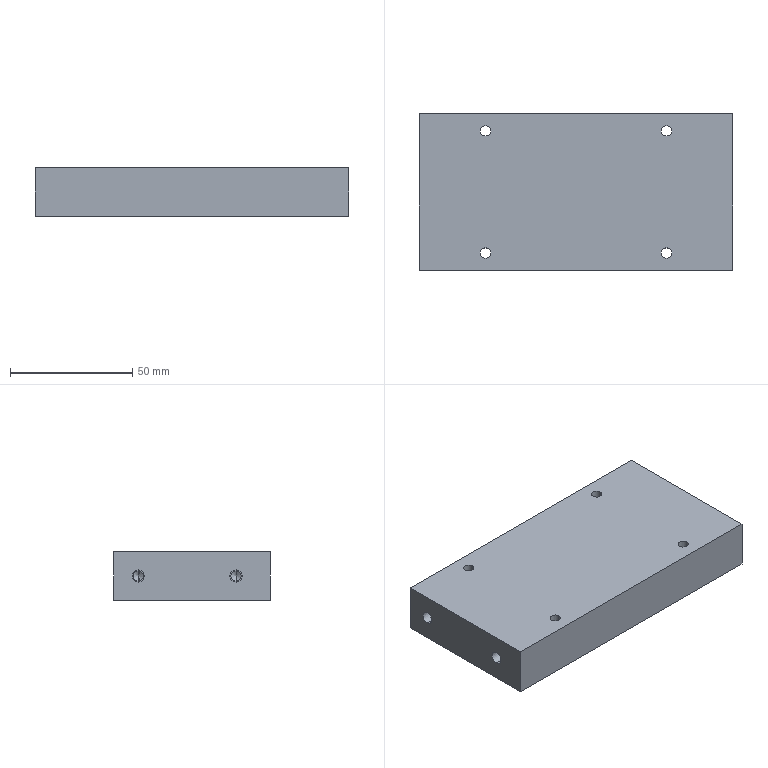Part | SolidWorks | features HoleWzd 2, MirrorPattern 2, Extrusion 1, LPattern 1 | 1 solid | 42 faces | box 128 x 64 x 20 mm | volume 161397 mm3 | cylinder 24 | plane 10 | cone 8 | commonest cylinder face diameters 4.2 x16 5 x8
STEP:
#1=CARTESIAN_POINT('',(109.338,14.,10.));
#2=VERTEX_POINT('',#1);
#3=CARTESIAN_POINT('',(110.6,14.,7.9));
#4=VERTEX_POINT('',#3);
#5=CARTESIAN_POINT('',(110.6,14.,7.9));
#6=DIRECTION('',(0.515,0.,-0.8572));
#7=VECTOR('',#6,1000.);
#8=LINE('',#5,#7);
#9=EDGE_CURVE('',#2,#4,#8,.T.);
#10=ORIENTED_EDGE('',*,*,#9,.F.);
#11=CARTESIAN_POINT('',(110.6,14.,12.1));
#12=VERTEX_POINT('',#11);
#13=CARTESIAN_POINT('',(110.6,14.,12.1));
#14=DIRECTION('',(0.515,0.,0.8572));
#15=VECTOR('',#14,1000.);
#16=LINE('',#13,#15);
#17=EDGE_CURVE('',#2,#12,#16,.T.);
#18=ORIENTED_EDGE('',*,*,#17,.T.);
#19=CARTESIAN_POINT('',(110.6,14.,10.));
#20=DIRECTION('',(1.,0.,0.));
#21=DIRECTION('',(0.,0.,-1.));
#22=AXIS2_PLACEMENT_3D('',#19,#20,#21);
#23=CIRCLE('',#22,2.1);
#24=EDGE_CURVE('',#12,#4,#23,.T.);
#25=ORIENTED_EDGE('',*,*,#24,.T.);
#26=EDGE_LOOP('',(#10,#18,#25));
#27=FACE_OUTER_BOUND('',#26,.T.);
#28=CARTESIAN_POINT('',(110.6,14.,10.));
#29=DIRECTION('',(1.,0.,0.));
#30=DIRECTION('',(0.,0.,-1.));
#31=AXIS2_PLACEMENT_3D('',#28,#29,#30);
#32=CONICAL_SURFACE('',#31,2.1,1.03);
#33=ADVANCED_FACE('',(#27),#32,.F.);
#34=ORIENTED_EDGE('',*,*,#24,.F.);
#35=CARTESIAN_POINT('',(113.,14.,12.1));
#36=VERTEX_POINT('',#35);
#37=CARTESIAN_POINT('',(128.,14.,12.1));
#38=DIRECTION('',(1.,0.,0.));
#39=VECTOR('',#38,1000.);
#40=LINE('',#37,#39);
#41=EDGE_CURVE('',#12,#36,#40,.T.);
#42=ORIENTED_EDGE('',*,*,#41,.T.);
#43=CARTESIAN_POINT('',(113.,14.,7.9));
#44=VERTEX_POINT('',#43);
#45=CARTESIAN_POINT('',(113.,14.,10.));
#46=DIRECTION('',(1.,0.,0.));
#47=DIRECTION('',(0.,0.,-1.));
#48=AXIS2_PLACEMENT_3D('',#45,#46,#47);
#49=CIRCLE('',#48,2.1);
#50=EDGE_CURVE('',#36,#44,#49,.T.);
#51=ORIENTED_EDGE('',*,*,#50,.T.);
#52=CARTESIAN_POINT('',(128.,14.,7.9));
#53=DIRECTION('',(1.,0.,0.));
#54=VECTOR('',#53,1000.);
#55=LINE('',#52,#54);
#56=EDGE_CURVE('',#4,#44,#55,.T.);
#57=ORIENTED_EDGE('',*,*,#56,.F.);
#58=EDGE_LOOP('',(#34,#42,#51,#57));
#59=FACE_OUTER_BOUND('',#58,.T.);
#60=CARTESIAN_POINT('',(128.,14.,10.));
#61=DIRECTION('',(1.,0.,0.));
#62=DIRECTION('',(0.,0.,-1.));
#63=AXIS2_PLACEMENT_3D('',#60,#61,#62);
#64=CYLINDRICAL_SURFACE('',#63,2.1);
#65=ADVANCED_FACE('',(#59),#64,.F.);
#66=CARTESIAN_POINT('',(113.,14.,12.5));
#67=VERTEX_POINT('',#66);
#68=CARTESIAN_POINT('',(113.,14.,7.5));
#69=VERTEX_POINT('',#68);
#70=CARTESIAN_POINT('',(113.,14.,10.));
#71=DIRECTION('',(1.,0.,0.));
#72=DIRECTION('',(0.,0.,-1.));
#73=AXIS2_PLACEMENT_3D('',#70,#71,#72);
#74=CIRCLE('',#73,2.5);
#75=EDGE_CURVE('',#67,#69,#74,.T.);
#76=ORIENTED_EDGE('',*,*,#75,.F.);
#77=CARTESIAN_POINT('',(128.,14.,12.5));
#78=VERTEX_POINT('',#77);
#79=CARTESIAN_POINT('',(128.,14.,12.5));
#80=DIRECTION('',(1.,0.,0.));
#81=VECTOR('',#80,1000.);
#82=LINE('',#79,#81);
#83=EDGE_CURVE('',#67,#78,#82,.T.);
#84=ORIENTED_EDGE('',*,*,#83,.T.);
#85=CARTESIAN_POINT('',(128.,14.,7.5));
#86=VERTEX_POINT('',#85);
#87=CARTESIAN_POINT('',(128.,14.,10.));
#88=DIRECTION('',(1.,0.,0.));
#89=DIRECTION('',(0.,0.,-1.));
#90=AXIS2_PLACEMENT_3D('',#87,#88,#89);
#91=CIRCLE('',#90,2.5);
#92=EDGE_CURVE('',#78,#86,#91,.T.);
#93=ORIENTED_EDGE('',*,*,#92,.T.);
#94=CARTESIAN_POINT('',(128.,14.,7.5));
#95=DIRECTION('',(1.,0.,0.));
#96=VECTOR('',#95,1000.);
#97=LINE('',#94,#96);
#98=EDGE_CURVE('',#69,#86,#97,.T.);
#99=ORIENTED_EDGE('',*,*,#98,.F.);
#100=EDGE_LOOP('',(#76,#84,#93,#99));
#101=FACE_OUTER_BOUND('',#100,.T.);
#102=CARTESIAN_POINT('',(128.,14.,10.));
#103=DIRECTION('',(1.,0.,0.));
#104=DIRECTION('',(0.,0.,-1.));
#105=AXIS2_PLACEMENT_3D('',#102,#103,#104);
#106=CYLINDRICAL_SURFACE('',#105,2.5);
#107=ADVANCED_FACE('',(#101),#106,.F.);
#108=CARTESIAN_POINT('',(18.662,14.,10.));
#109=VERTEX_POINT('',#108);
#110=CARTESIAN_POINT('',(17.4,14.,12.1));
#111=VERTEX_POINT('',#110);
#112=CARTESIAN_POINT('',(17.4,14.,12.1));
#113=DIRECTION('',(-0.515,0.,0.8572));
#114=VECTOR('',#113,1000.);
#115=LINE('',#112,#114);
#116=EDGE_CURVE('',#109,#111,#115,.T.);
#117=ORIENTED_EDGE('',*,*,#116,.F.);
#118=CARTESIAN_POINT('',(17.4,14.,7.9));
#119=VERTEX_POINT('',#118);
#120=CARTESIAN_POINT('',(17.4,14.,7.9));
#121=DIRECTION('',(-0.515,0.,-0.8572));
#122=VECTOR('',#121,1000.);
#123=LINE('',#120,#122);
#124=EDGE_CURVE('',#109,#119,#123,.T.);
#125=ORIENTED_EDGE('',*,*,#124,.T.);
#126=CARTESIAN_POINT('',(17.4,14.,10.));
#127=DIRECTION('',(-1.,0.,0.));
#128=DIRECTION('',(0.,0.,1.));
#129=AXIS2_PLACEMENT_3D('',#126,#127,#128);
#130=CIRCLE('',#129,2.1);
#131=EDGE_CURVE('',#119,#111,#130,.T.);
#132=ORIENTED_EDGE('',*,*,#131,.T.);
#133=EDGE_LOOP('',(#117,#125,#132));
#134=FACE_OUTER_BOUND('',#133,.T.);
#135=CARTESIAN_POINT('',(17.4,14.,10.));
#136=DIRECTION('',(-1.,0.,0.));
#137=DIRECTION('',(0.,0.,1.));
#138=AXIS2_PLACEMENT_3D('',#135,#136,#137);
#139=CONICAL_SURFACE('',#138,2.1,1.03);
#140=ADVANCED_FACE('',(#134),#139,.F.);
#141=ORIENTED_EDGE('',*,*,#131,.F.);
#142=CARTESIAN_POINT('',(15.,14.,7.9));
#143=VERTEX_POINT('',#142);
#144=CARTESIAN_POINT('',(0.,14.,7.9));
#145=DIRECTION('',(-1.,0.,0.));
#146=VECTOR('',#145,1000.);
#147=LINE('',#144,#146);
#148=EDGE_CURVE('',#119,#143,#147,.T.);
#149=ORIENTED_EDGE('',*,*,#148,.T.);
#150=CARTESIAN_POINT('',(15.,14.,12.1));
#151=VERTEX_POINT('',#150);
#152=CARTESIAN_POINT('',(15.,14.,10.));
#153=DIRECTION('',(-1.,0.,0.));
#154=DIRECTION('',(0.,0.,1.));
#155=AXIS2_PLACEMENT_3D('',#152,#153,#154);
#156=CIRCLE('',#155,2.1);
#157=EDGE_CURVE('',#143,#151,#156,.T.);
#158=ORIENTED_EDGE('',*,*,#157,.T.);
#159=CARTESIAN_POINT('',(0.,14.,12.1));
#160=DIRECTION('',(-1.,0.,0.));
#161=VECTOR('',#160,1000.);
#162=LINE('',#159,#161);
#163=EDGE_CURVE('',#111,#151,#162,.T.);
#164=ORIENTED_EDGE('',*,*,#163,.F.);
#165=EDGE_LOOP('',(#141,#149,#158,#164));
#166=FACE_OUTER_BOUND('',#165,.T.);
#167=CARTESIAN_POINT('',(0.,14.,10.));
#168=DIRECTION('',(-1.,0.,0.));
#169=DIRECTION('',(0.,0.,1.));
#170=AXIS2_PLACEMENT_3D('',#167,#168,#169);
#171=CYLINDRICAL_SURFACE('',#170,2.1);
#172=ADVANCED_FACE('',(#166),#171,.F.);
#173=CARTESIAN_POINT('',(15.,14.,7.5));
#174=VERTEX_POINT('',#173);
#175=CARTESIAN_POINT('',(15.,14.,12.5));
#176=VERTEX_POINT('',#175);
#177=CARTESIAN_POINT('',(15.,14.,10.));
#178=DIRECTION('',(-1.,0.,0.));
#179=DIRECTION('',(0.,0.,1.));
#180=AXIS2_PLACEMENT_3D('',#177,#178,#179);
#181=CIRCLE('',#180,2.5);
#182=EDGE_CURVE('',#174,#176,#181,.T.);
#183=ORIENTED_EDGE('',*,*,#182,.F.);
#184=CARTESIAN_POINT('',(0.,14.,7.5));
#185=VERTEX_POINT('',#184);
#186=CARTESIAN_POINT('',(0.,14.,7.5));
#187=DIRECTION('',(-1.,0.,0.));
#188=VECTOR('',#187,1000.);
#189=LINE('',#186,#188);
#190=EDGE_CURVE('',#174,#185,#189,.T.);
#191=ORIENTED_EDGE('',*,*,#190,.T.);
#192=CARTESIAN_POINT('',(0.,14.,12.5));
#193=VERTEX_POINT('',#192);
#194=CARTESIAN_POINT('',(0.,14.,10.));
#195=DIRECTION('',(-1.,0.,0.));
#196=DIRECTION('',(0.,0.,1.));
#197=AXIS2_PLACEMENT_3D('',#194,#195,#196);
#198=CIRCLE('',#197,2.5);
#199=EDGE_CURVE('',#185,#193,#198,.T.);
#200=ORIENTED_EDGE('',*,*,#199,.T.);
#201=CARTESIAN_POINT('',(0.,14.,12.5));
#202=DIRECTION('',(-1.,0.,0.));
#203=VECTOR('',#202,1000.);
#204=LINE('',#201,#203);
#205=EDGE_CURVE('',#176,#193,#204,.T.);
#206=ORIENTED_EDGE('',*,*,#205,.F.);
#207=EDGE_LOOP('',(#183,#191,#200,#206));
#208=FACE_OUTER_BOUND('',#207,.T.);
#209=CARTESIAN_POINT('',(0.,14.,10.));
#210=DIRECTION('',(-1.,0.,0.));
#211=DIRECTION('',(0.,0.,1.));
#212=AXIS2_PLACEMENT_3D('',#209,#210,#211);
#213=CYLINDRICAL_SURFACE('',#212,2.5);
#214=ADVANCED_FACE('',(#208),#213,.F.);
#215=CARTESIAN_POINT('',(109.338,54.,10.));
#216=VERTEX_POINT('',#215);
#217=CARTESIAN_POINT('',(110.6,54.,7.9));
#218=VERTEX_POINT('',#217);
#219=CARTESIAN_POINT('',(110.6,54.,7.9));
#220=DIRECTION('',(0.515,0.,-0.8572));
#221=VECTOR('',#220,1000.);
#222=LINE('',#219,#221);
#223=EDGE_CURVE('',#216,#218,#222,.T.);
#224=ORIENTED_EDGE('',*,*,#223,.F.);
#225=CARTESIAN_POINT('',(110.6,54.,12.1));
#226=VERTEX_POINT('',#225);
#227=CARTESIAN_POINT('',(110.6,54.,12.1));
#228=DIRECTION('',(0.515,0.,0.8572));
#229=VECTOR('',#228,1000.);
#230=LINE('',#227,#229);
#231=EDGE_CURVE('',#216,#226,#230,.T.);
#232=ORIENTED_EDGE('',*,*,#231,.T.);
#233=CARTESIAN_POINT('',(110.6,54.,10.));
#234=DIRECTION('',(1.,0.,0.));
#235=DIRECTION('',(0.,0.,-1.));
#236=AXIS2_PLACEMENT_3D('',#233,#234,#235);
#237=CIRCLE('',#236,2.1);
#238=EDGE_CURVE('',#226,#218,#237,.T.);
#239=ORIENTED_EDGE('',*,*,#238,.T.);
#240=EDGE_LOOP('',(#224,#232,#239));
#241=FACE_OUTER_BOUND('',#240,.T.);
#242=CARTESIAN_POINT('',(110.6,54.,10.));
#243=DIRECTION('',(1.,0.,0.));
#244=DIRECTION('',(0.,0.,-1.));
#245=AXIS2_PLACEMENT_3D('',#242,#243,#244);
#246=CONICAL_SURFACE('',#245,2.1,1.03);
#247=ADVANCED_FACE('',(#241),#246,.F.);
#248=ORIENTED_EDGE('',*,*,#238,.F.);
#249=CARTESIAN_POINT('',(113.,54.,12.1));
#250=VERTEX_POINT('',#249);
#251=CARTESIAN_POINT('',(128.,54.,12.1));
#252=DIRECTION('',(1.,0.,0.));
#253=VECTOR('',#252,1000.);
#254=LINE('',#251,#253);
#255=EDGE_CURVE('',#226,#250,#254,.T.);
#256=ORIENTED_EDGE('',*,*,#255,.T.);
#257=CARTESIAN_POINT('',(113.,54.,7.9));
#258=VERTEX_POINT('',#257);
#259=CARTESIAN_POINT('',(113.,54.,10.));
#260=DIRECTION('',(1.,0.,0.));
#261=DIRECTION('',(0.,0.,-1.));
#262=AXIS2_PLACEMENT_3D('',#259,#260,#261);
#263=CIRCLE('',#262,2.1);
#264=EDGE_CURVE('',#250,#258,#263,.T.);
#265=ORIENTED_EDGE('',*,*,#264,.T.);
#266=CARTESIAN_POINT('',(128.,54.,7.9));
#267=DIRECTION('',(1.,0.,0.));
#268=VECTOR('',#267,1000.);
#269=LINE('',#266,#268);
#270=EDGE_CURVE('',#218,#258,#269,.T.);
#271=ORIENTED_EDGE('',*,*,#270,.F.);
#272=EDGE_LOOP('',(#248,#256,#265,#271));
#273=FACE_OUTER_BOUND('',#272,.T.);
#274=CARTESIAN_POINT('',(128.,54.,10.));
#275=DIRECTION('',(1.,0.,0.));
#276=DIRECTION('',(0.,0.,-1.));
#277=AXIS2_PLACEMENT_3D('',#274,#275,#276);
#278=CYLINDRICAL_SURFACE('',#277,2.1);
#279=ADVANCED_FACE('',(#273),#278,.F.);
#280=CARTESIAN_POINT('',(113.,54.,12.5));
#281=VERTEX_POINT('',#280);
#282=CARTESIAN_POINT('',(113.,54.,7.5));
#283=VERTEX_POINT('',#282);
#284=CARTESIAN_POINT('',(113.,54.,10.));
#285=DIRECTION('',(1.,0.,0.));
#286=DIRECTION('',(0.,0.,-1.));
#287=AXIS2_PLACEMENT_3D('',#284,#285,#286);
#288=CIRCLE('',#287,2.5);
#289=EDGE_CURVE('',#281,#283,#288,.T.);
#290=ORIENTED_EDGE('',*,*,#289,.F.);
#291=CARTESIAN_POINT('',(128.,54.,12.5));
#292=VERTEX_POINT('',#291);
#293=CARTESIAN_POINT('',(128.,54.,12.5));
#294=DIRECTION('',(1.,0.,0.));
#295=VECTOR('',#294,1000.);
#296=LINE('',#293,#295);
#297=EDGE_CURVE('',#281,#292,#296,.T.);
#298=ORIENTED_EDGE('',*,*,#297,.T.);
#299=CARTESIAN_POINT('',(128.,54.,7.5));
#300=VERTEX_POINT('',#299);
#301=CARTESIAN_POINT('',(128.,54.,10.));
#302=DIRECTION('',(1.,0.,0.));
#303=DIRECTION('',(0.,0.,-1.));
#304=AXIS2_PLACEMENT_3D('',#301,#302,#303);
#305=CIRCLE('',#304,2.5);
#306=EDGE_CURVE('',#292,#300,#305,.T.);
#307=ORIENTED_EDGE('',*,*,#306,.T.);
#308=CARTESIAN_POINT('',(128.,54.,7.5));
#309=DIRECTION('',(1.,0.,0.));
#310=VECTOR('',#309,1000.);
#311=LINE('',#308,#310);
#312=EDGE_CURVE('',#283,#300,#311,.T.);
#313=ORIENTED_EDGE('',*,*,#312,.F.);
#314=EDGE_LOOP('',(#290,#298,#307,#313));
#315=FACE_OUTER_BOUND('',#314,.T.);
#316=CARTESIAN_POINT('',(128.,54.,10.));
#317=DIRECTION('',(1.,0.,0.));
#318=DIRECTION('',(0.,0.,-1.));
#319=AXIS2_PLACEMENT_3D('',#316,#317,#318);
#320=CYLINDRICAL_SURFACE('',#319,2.5);
#321=ADVANCED_FACE('',(#315),#320,.F.);
#322=CARTESIAN_POINT('',(18.662,54.,10.));
#323=VERTEX_POINT('',#322);
#324=CARTESIAN_POINT('',(17.4,54.,12.1));
#325=VERTEX_POINT('',#324);
#326=CARTESIAN_POINT('',(17.4,54.,12.1));
#327=DIRECTION('',(-0.515,0.,0.8572));
#328=VECTOR('',#327,1000.);
#329=LINE('',#326,#328);
#330=EDGE_CURVE('',#323,#325,#329,.T.);
#331=ORIENTED_EDGE('',*,*,#330,.F.);
#332=CARTESIAN_POINT('',(17.4,54.,7.9));
#333=VERTEX_POINT('',#332);
#334=CARTESIAN_POINT('',(17.4,54.,7.9));
#335=DIRECTION('',(-0.515,0.,-0.8572));
#336=VECTOR('',#335,1000.);
#337=LINE('',#334,#336);
#338=EDGE_CURVE('',#323,#333,#337,.T.);
#339=ORIENTED_EDGE('',*,*,#338,.T.);
#340=CARTESIAN_POINT('',(17.4,54.,10.));
#341=DIRECTION('',(-1.,0.,0.));
#342=DIRECTION('',(0.,0.,1.));
#343=AXIS2_PLACEMENT_3D('',#340,#341,#342);
#344=CIRCLE('',#343,2.1);
#345=EDGE_CURVE('',#333,#325,#344,.T.);
#346=ORIENTED_EDGE('',*,*,#345,.T.);
#347=EDGE_LOOP('',(#331,#339,#346));
#348=FACE_OUTER_BOUND('',#347,.T.);
#349=CARTESIAN_POINT('',(17.4,54.,10.));
#350=DIRECTION('',(-1.,0.,0.));
#351=DIRECTION('',(0.,0.,1.));
#352=AXIS2_PLACEMENT_3D('',#349,#350,#351);
#353=CONICAL_SURFACE('',#352,2.1,1.03);
#354=ADVANCED_FACE('',(#348),#353,.F.);
#355=ORIENTED_EDGE('',*,*,#345,.F.);
#356=CARTESIAN_POINT('',(15.,54.,7.9));
#357=VERTEX_POINT('',#356);
#358=CARTESIAN_POINT('',(0.,54.,7.9));
#359=DIRECTION('',(-1.,0.,0.));
#360=VECTOR('',#359,1000.);
#361=LINE('',#358,#360);
#362=EDGE_CURVE('',#333,#357,#361,.T.);
#363=ORIENTED_EDGE('',*,*,#362,.T.);
#364=CARTESIAN_POINT('',(15.,54.,12.1));
#365=VERTEX_POINT('',#364);
#366=CARTESIAN_POINT('',(15.,54.,10.));
#367=DIRECTION('',(-1.,0.,0.));
#368=DIRECTION('',(0.,0.,1.));
#369=AXIS2_PLACEMENT_3D('',#366,#367,#368);
#370=CIRCLE('',#369,2.1);
#371=EDGE_CURVE('',#357,#365,#370,.T.);
#372=ORIENTED_EDGE('',*,*,#371,.T.);
#373=CARTESIAN_POINT('',(0.,54.,12.1));
#374=DIRECTION('',(-1.,0.,0.));
#375=VECTOR('',#374,1000.);
#376=LINE('',#373,#375);
#377=EDGE_CURVE('',#325,#365,#376,.T.);
#378=ORIENTED_EDGE('',*,*,#377,.F.);
#379=EDGE_LOOP('',(#355,#363,#372,#378));
#380=FACE_OUTER_BOUND('',#379,.T.);
#381=CARTESIAN_POINT('',(0.,54.,10.));
#382=DIRECTION('',(-1.,0.,0.));
#383=DIRECTION('',(0.,0.,1.));
#384=AXIS2_PLACEMENT_3D('',#381,#382,#383);
#385=CYLINDRICAL_SURFACE('',#384,2.1);
#386=ADVANCED_FACE('',(#380),#385,.F.);
#387=CARTESIAN_POINT('',(15.,54.,7.5));
#388=VERTEX_POINT('',#387);
#389=CARTESIAN_POINT('',(15.,54.,12.5));
#390=VERTEX_POINT('',#389);
#391=CARTESIAN_POINT('',(15.,54.,10.));
#392=DIRECTION('',(-1.,0.,0.));
#393=DIRECTION('',(0.,0.,1.));
#394=AXIS2_PLACEMENT_3D('',#391,#392,#393);
#395=CIRCLE('',#394,2.5);
#396=EDGE_CURVE('',#388,#390,#395,.T.);
#397=ORIENTED_EDGE('',*,*,#396,.F.);
#398=CARTESIAN_POINT('',(0.,54.,7.5));
#399=VERTEX_POINT('',#398);
#400=CARTESIAN_POINT('',(0.,54.,7.5));
#401=DIRECTION('',(-1.,0.,0.));
#402=VECTOR('',#401,1000.);
#403=LINE('',#400,#402);
#404=EDGE_CURVE('',#388,#399,#403,.T.);
#405=ORIENTED_EDGE('',*,*,#404,.T.);
#406=CARTESIAN_POINT('',(0.,54.,12.5));
#407=VERTEX_POINT('',#406);
#408=CARTESIAN_POINT('',(0.,54.,10.));
#409=DIRECTION('',(-1.,0.,0.));
#410=DIRECTION('',(0.,0.,1.));
#411=AXIS2_PLACEMENT_3D('',#408,#409,#410);
#412=CIRCLE('',#411,2.5);
#413=EDGE_CURVE('',#399,#407,#412,.T.);
#414=ORIENTED_EDGE('',*,*,#413,.T.);
#415=CARTESIAN_POINT('',(0.,54.,12.5));
#416=DIRECTION('',(-1.,0.,0.));
#417=VECTOR('',#416,1000.);
#418=LINE('',#415,#417);
#419=EDGE_CURVE('',#390,#407,#418,.T.);
#420=ORIENTED_EDGE('',*,*,#419,.F.);
#421=EDGE_LOOP('',(#397,#405,#414,#420));
#422=FACE_OUTER_BOUND('',#421,.T.);
#423=CARTESIAN_POINT('',(0.,54.,10.));
#424=DIRECTION('',(-1.,0.,0.));
#425=DIRECTION('',(0.,0.,1.));
#426=AXIS2_PLACEMENT_3D('',#423,#424,#425);
#427=CYLINDRICAL_SURFACE('',#426,2.5);
#428=ADVANCED_FACE('',(#422),#427,.F.);
#429=CARTESIAN_POINT('',(24.9,57.,0.));
#430=VERTEX_POINT('',#429);
#431=CARTESIAN_POINT('',(29.1,57.,0.));
#432=VERTEX_POINT('',#431);
#433=CARTESIAN_POINT('',(27.,57.,0.));
#434=DIRECTION('',(0.,0.,1.));
#435=DIRECTION('',(1.,0.,0.));
#436=AXIS2_PLACEMENT_3D('',#433,#434,#435);
#437=CIRCLE('',#436,2.1);
#438=EDGE_CURVE('',#430,#432,#437,.T.);
#439=ORIENTED_EDGE('',*,*,#438,.F.);
#440=CARTESIAN_POINT('',(24.9,57.,20.));
#441=VERTEX_POINT('',#440);
#442=CARTESIAN_POINT('',(24.9,57.,20.));
#443=DIRECTION('',(0.,0.,1.));
#444=VECTOR('',#443,1000.);
#445=LINE('',#442,#444);
#446=EDGE_CURVE('',#430,#441,#445,.T.);
#447=ORIENTED_EDGE('',*,*,#446,.T.);
#448=CARTESIAN_POINT('',(29.1,57.,20.));
#449=VERTEX_POINT('',#448);
#450=CARTESIAN_POINT('',(27.,57.,20.));
#451=DIRECTION('',(0.,0.,1.));
#452=DIRECTION('',(1.,0.,0.));
#453=AXIS2_PLACEMENT_3D('',#450,#451,#452);
#454=CIRCLE('',#453,2.1);
#455=EDGE_CURVE('',#441,#449,#454,.T.);
#456=ORIENTED_EDGE('',*,*,#455,.T.);
#457=CARTESIAN_POINT('',(29.1,57.,20.));
#458=DIRECTION('',(0.,0.,1.));
#459=VECTOR('',#458,1000.);
#460=LINE('',#457,#459);
#461=EDGE_CURVE('',#432,#449,#460,.T.);
#462=ORIENTED_EDGE('',*,*,#461,.F.);
#463=EDGE_LOOP('',(#439,#447,#456,#462));
#464=FACE_OUTER_BOUND('',#463,.T.);
#465=CARTESIAN_POINT('',(27.,57.,20.));
#466=DIRECTION('',(0.,0.,1.));
#467=DIRECTION('',(1.,0.,0.));
#468=AXIS2_PLACEMENT_3D('',#465,#466,#467);
#469=CYLINDRICAL_SURFACE('',#468,2.1);
#470=ADVANCED_FACE('',(#464),#469,.F.);
#471=CARTESIAN_POINT('',(24.9,7.,0.));
#472=VERTEX_POINT('',#471);
#473=CARTESIAN_POINT('',(29.1,7.,0.));
#474=VERTEX_POINT('',#473);
#475=CARTESIAN_POINT('',(27.,7.,0.));
#476=DIRECTION('',(0.,0.,1.));
#477=DIRECTION('',(1.,0.,0.));
#478=AXIS2_PLACEMENT_3D('',#475,#476,#477);
#479=CIRCLE('',#478,2.1);
#480=EDGE_CURVE('',#472,#474,#479,.T.);
#481=ORIENTED_EDGE('',*,*,#480,.F.);
#482=CARTESIAN_POINT('',(24.9,7.,20.));
#483=VERTEX_POINT('',#482);
#484=CARTESIAN_POINT('',(24.9,7.,20.));
#485=DIRECTION('',(0.,0.,1.));
#486=VECTOR('',#485,1000.);
#487=LINE('',#484,#486);
#488=EDGE_CURVE('',#472,#483,#487,.T.);
#489=ORIENTED_EDGE('',*,*,#488,.T.);
#490=CARTESIAN_POINT('',(29.1,7.,20.));
#491=VERTEX_POINT('',#490);
#492=CARTESIAN_POINT('',(27.,7.,20.));
#493=DIRECTION('',(0.,0.,1.));
#494=DIRECTION('',(1.,0.,0.));
#495=AXIS2_PLACEMENT_3D('',#492,#493,#494);
#496=CIRCLE('',#495,2.1);
#497=EDGE_CURVE('',#483,#491,#496,.T.);
#498=ORIENTED_EDGE('',*,*,#497,.T.);
#499=CARTESIAN_POINT('',(29.1,7.,20.));
#500=DIRECTION('',(0.,0.,1.));
#501=VECTOR('',#500,1000.);
#502=LINE('',#499,#501);
#503=EDGE_CURVE('',#474,#491,#502,.T.);
#504=ORIENTED_EDGE('',*,*,#503,.F.);
#505=EDGE_LOOP('',(#481,#489,#498,#504));
#506=FACE_OUTER_BOUND('',#505,.T.);
#507=CARTESIAN_POINT('',(27.,7.,20.));
#508=DIRECTION('',(0.,0.,1.));
#509=DIRECTION('',(1.,0.,0.));
#510=AXIS2_PLACEMENT_3D('',#507,#508,#509);
#511=CYLINDRICAL_SURFACE('',#510,2.1);
#512=ADVANCED_FACE('',(#506),#511,.F.);
#513=CARTESIAN_POINT('',(98.9,7.,0.));
#514=VERTEX_POINT('',#513);
#515=CARTESIAN_POINT('',(103.1,7.,0.));
#516=VERTEX_POINT('',#515);
#517=CARTESIAN_POINT('',(101.,7.,0.));
#518=DIRECTION('',(0.,0.,1.));
#519=DIRECTION('',(1.,0.,0.));
#520=AXIS2_PLACEMENT_3D('',#517,#518,#519);
#521=CIRCLE('',#520,2.1);
#522=EDGE_CURVE('',#514,#516,#521,.T.);
#523=ORIENTED_EDGE('',*,*,#522,.F.);
#524=CARTESIAN_POINT('',(98.9,7.,20.));
#525=VERTEX_POINT('',#524);
#526=CARTESIAN_POINT('',(98.9,7.,20.));
#527=DIRECTION('',(0.,0.,1.));
#528=VECTOR('',#527,1000.);
#529=LINE('',#526,#528);
#530=EDGE_CURVE('',#514,#525,#529,.T.);
#531=ORIENTED_EDGE('',*,*,#530,.T.);
#532=CARTESIAN_POINT('',(103.1,7.,20.));
#533=VERTEX_POINT('',#532);
#534=CARTESIAN_POINT('',(101.,7.,20.));
#535=DIRECTION('',(0.,0.,1.));
#536=DIRECTION('',(1.,0.,0.));
#537=AXIS2_PLACEMENT_3D('',#534,#535,#536);
#538=CIRCLE('',#537,2.1);
#539=EDGE_CURVE('',#525,#533,#538,.T.);
#540=ORIENTED_EDGE('',*,*,#539,.T.);
#541=CARTESIAN_POINT('',(103.1,7.,20.));
#542=DIRECTION('',(0.,0.,1.));
#543=VECTOR('',#542,1000.);
#544=LINE('',#541,#543);
#545=EDGE_CURVE('',#516,#533,#544,.T.);
#546=ORIENTED_EDGE('',*,*,#545,.F.);
#547=EDGE_LOOP('',(#523,#531,#540,#546));
#548=FACE_OUTER_BOUND('',#547,.T.);
#549=CARTESIAN_POINT('',(101.,7.,20.));
#550=DIRECTION('',(0.,0.,1.));
#551=DIRECTION('',(1.,0.,0.));
#552=AXIS2_PLACEMENT_3D('',#549,#550,#551);
#553=CYLINDRICAL_SURFACE('',#552,2.1);
#554=ADVANCED_FACE('',(#548),#553,.F.);
#555=CARTESIAN_POINT('',(98.9,57.,0.));
#556=VERTEX_POINT('',#555);
#557=CARTESIAN_POINT('',(103.1,57.,0.));
#558=VERTEX_POINT('',#557);
#559=CARTESIAN_POINT('',(101.,57.,0.));
#560=DIRECTION('',(0.,0.,1.));
#561=DIRECTION('',(1.,0.,0.));
#562=AXIS2_PLACEMENT_3D('',#559,#560,#561);
#563=CIRCLE('',#562,2.1);
#564=EDGE_CURVE('',#556,#558,#563,.T.);
#565=ORIENTED_EDGE('',*,*,#564,.F.);
#566=CARTESIAN_POINT('',(98.9,57.,20.));
#567=VERTEX_POINT('',#566);
#568=CARTESIAN_POINT('',(98.9,57.,20.));
#569=DIRECTION('',(0.,0.,1.));
#570=VECTOR('',#569,1000.);
#571=LINE('',#568,#570);
#572=EDGE_CURVE('',#556,#567,#571,.T.);
#573=ORIENTED_EDGE('',*,*,#572,.T.);
#574=CARTESIAN_POINT('',(103.1,57.,20.));
#575=VERTEX_POINT('',#574);
#576=CARTESIAN_POINT('',(101.,57.,20.));
#577=DIRECTION('',(0.,0.,1.));
#578=DIRECTION('',(1.,0.,0.));
#579=AXIS2_PLACEMENT_3D('',#576,#577,#578);
#580=CIRCLE('',#579,2.1);
#581=EDGE_CURVE('',#567,#575,#580,.T.);
#582=ORIENTED_EDGE('',*,*,#581,.T.);
#583=CARTESIAN_POINT('',(103.1,57.,20.));
#584=DIRECTION('',(0.,0.,1.));
#585=VECTOR('',#584,1000.);
#586=LINE('',#583,#585);
#587=EDGE_CURVE('',#558,#575,#586,.T.);
#588=ORIENTED_EDGE('',*,*,#587,.F.);
#589=EDGE_LOOP('',(#565,#573,#582,#588));
#590=FACE_OUTER_BOUND('',#589,.T.);
#591=CARTESIAN_POINT('',(101.,57.,20.));
#592=DIRECTION('',(0.,0.,1.));
#593=DIRECTION('',(1.,0.,0.));
#594=AXIS2_PLACEMENT_3D('',#591,#592,#593);
#595=CYLINDRICAL_SURFACE('',#594,2.1);
#596=ADVANCED_FACE('',(#590),#595,.F.);
#597=CARTESIAN_POINT('',(27.,57.,0.));
#598=DIRECTION('',(0.,0.,1.));
#599=DIRECTION('',(1.,0.,0.));
#600=AXIS2_PLACEMENT_3D('',#597,#598,#599);
#601=CIRCLE('',#600,2.1);
#602=EDGE_CURVE('',#432,#430,#601,.T.);
#603=ORIENTED_EDGE('',*,*,#602,.T.);
#604=ORIENTED_EDGE('',*,*,#438,.T.);
#605=EDGE_LOOP('',(#603,#604));
#606=FACE_BOUND('',#605,.T.);
#607=CARTESIAN_POINT('',(27.,7.,0.));
#608=DIRECTION('',(0.,0.,1.));
#609=DIRECTION('',(1.,0.,0.));
#610=AXIS2_PLACEMENT_3D('',#607,#608,#609);
#611=CIRCLE('',#610,2.1);
#612=EDGE_CURVE('',#474,#472,#611,.T.);
#613=ORIENTED_EDGE('',*,*,#612,.T.);
#614=ORIENTED_EDGE('',*,*,#480,.T.);
#615=EDGE_LOOP('',(#613,#614));
#616=FACE_BOUND('',#615,.T.);
#617=CARTESIAN_POINT('',(101.,7.,0.));
#618=DIRECTION('',(0.,0.,1.));
#619=DIRECTION('',(1.,0.,0.));
#620=AXIS2_PLACEMENT_3D('',#617,#618,#619);
#621=CIRCLE('',#620,2.1);
#622=EDGE_CURVE('',#516,#514,#621,.T.);
#623=ORIENTED_EDGE('',*,*,#622,.T.);
#624=ORIENTED_EDGE('',*,*,#522,.T.);
#625=EDGE_LOOP('',(#623,#624));
#626=FACE_BOUND('',#625,.T.);
#627=CARTESIAN_POINT('',(0.,64.,0.));
#628=VERTEX_POINT('',#627);
#629=CARTESIAN_POINT('',(0.,0.,0.));
#630=VERTEX_POINT('',#629);
#631=CARTESIAN_POINT('',(0.,0.,0.));
#632=DIRECTION('',(0.,-1.,0.));
#633=VECTOR('',#632,1000.);
#634=LINE('',#631,#633);
#635=EDGE_CURVE('',#628,#630,#634,.T.);
#636=ORIENTED_EDGE('',*,*,#635,.F.);
#637=CARTESIAN_POINT('',(128.,64.,0.));
#638=VERTEX_POINT('',#637);
#639=CARTESIAN_POINT('',(0.,64.,0.));
#640=DIRECTION('',(-1.,0.,0.));
#641=VECTOR('',#640,1000.);
#642=LINE('',#639,#641);
#643=EDGE_CURVE('',#638,#628,#642,.T.);
#644=ORIENTED_EDGE('',*,*,#643,.F.);
#645=CARTESIAN_POINT('',(128.,0.,0.));
#646=VERTEX_POINT('',#645);
#647=CARTESIAN_POINT('',(128.,0.,0.));
#648=DIRECTION('',(0.,1.,0.));
#649=VECTOR('',#648,1000.);
#650=LINE('',#647,#649);
#651=EDGE_CURVE('',#646,#638,#650,.T.);
#652=ORIENTED_EDGE('',*,*,#651,.F.);
#653=CARTESIAN_POINT('',(0.,0.,0.));
#654=DIRECTION('',(1.,0.,0.));
#655=VECTOR('',#654,1000.);
#656=LINE('',#653,#655);
#657=EDGE_CURVE('',#630,#646,#656,.T.);
#658=ORIENTED_EDGE('',*,*,#657,.F.);
#659=EDGE_LOOP('',(#636,#644,#652,#658));
#660=FACE_OUTER_BOUND('',#659,.T.);
#661=CARTESIAN_POINT('',(101.,57.,0.));
#662=DIRECTION('',(0.,0.,1.));
#663=DIRECTION('',(1.,0.,0.));
#664=AXIS2_PLACEMENT_3D('',#661,#662,#663);
#665=CIRCLE('',#664,2.1);
#666=EDGE_CURVE('',#558,#556,#665,.T.);
#667=ORIENTED_EDGE('',*,*,#666,.T.);
#668=ORIENTED_EDGE('',*,*,#564,.T.);
#669=EDGE_LOOP('',(#667,#668));
#670=FACE_BOUND('',#669,.T.);
#671=CARTESIAN_POINT('',(0.,64.,0.));
#672=DIRECTION('',(0.,0.,-1.));
#673=DIRECTION('',(-1.,0.,0.));
#674=AXIS2_PLACEMENT_3D('',#671,#672,#673);
#675=PLANE('',#674);
#676=ADVANCED_FACE('',(#606,#616,#626,#660,#670),#675,.T.);
#677=CARTESIAN_POINT('',(0.,14.,10.));
#678=DIRECTION('',(-1.,0.,0.));
#679=DIRECTION('',(0.,0.,1.));
#680=AXIS2_PLACEMENT_3D('',#677,#678,#679);
#681=CIRCLE('',#680,2.5);
#682=EDGE_CURVE('',#193,#185,#681,.T.);
#683=ORIENTED_EDGE('',*,*,#682,.F.);
#684=ORIENTED_EDGE('',*,*,#199,.F.);
#685=EDGE_LOOP('',(#683,#684));
#686=FACE_BOUND('',#685,.T.);
#687=CARTESIAN_POINT('',(0.,54.,10.));
#688=DIRECTION('',(-1.,0.,0.));
#689=DIRECTION('',(0.,0.,1.));
#690=AXIS2_PLACEMENT_3D('',#687,#688,#689);
#691=CIRCLE('',#690,2.5);
#692=EDGE_CURVE('',#407,#399,#691,.T.);
#693=ORIENTED_EDGE('',*,*,#692,.F.);
#694=ORIENTED_EDGE('',*,*,#413,.F.);
#695=EDGE_LOOP('',(#693,#694));
#696=FACE_BOUND('',#695,.T.);
#697=ORIENTED_EDGE('',*,*,#635,.T.);
#698=CARTESIAN_POINT('',(0.,0.,20.));
#699=VERTEX_POINT('',#698);
#700=CARTESIAN_POINT('',(0.,0.,20.));
#701=DIRECTION('',(0.,0.,-1.));
#702=VECTOR('',#701,1000.);
#703=LINE('',#700,#702);
#704=EDGE_CURVE('',#699,#630,#703,.T.);
#705=ORIENTED_EDGE('',*,*,#704,.F.);
#706=CARTESIAN_POINT('',(0.,64.,20.));
#707=VERTEX_POINT('',#706);
#708=CARTESIAN_POINT('',(0.,0.,20.));
#709=DIRECTION('',(0.,-1.,0.));
#710=VECTOR('',#709,1000.);
#711=LINE('',#708,#710);
#712=EDGE_CURVE('',#707,#699,#711,.T.);
#713=ORIENTED_EDGE('',*,*,#712,.F.);
#714=CARTESIAN_POINT('',(0.,64.,20.));
#715=DIRECTION('',(0.,0.,-1.));
#716=VECTOR('',#715,1000.);
#717=LINE('',#714,#716);
#718=EDGE_CURVE('',#707,#628,#717,.T.);
#719=ORIENTED_EDGE('',*,*,#718,.T.);
#720=EDGE_LOOP('',(#697,#705,#713,#719));
#721=FACE_OUTER_BOUND('',#720,.T.);
#722=CARTESIAN_POINT('',(0.,0.,20.));
#723=DIRECTION('',(1.,0.,0.));
#724=DIRECTION('',(0.,0.,-1.));
#725=AXIS2_PLACEMENT_3D('',#722,#723,#724);
#726=PLANE('',#725);
#727=ADVANCED_FACE('',(#686,#696,#721),#726,.F.);
#728=ORIENTED_EDGE('',*,*,#657,.T.);
#729=CARTESIAN_POINT('',(128.,0.,20.));
#730=VERTEX_POINT('',#729);
#731=CARTESIAN_POINT('',(128.,0.,20.));
#732=DIRECTION('',(0.,0.,-1.));
#733=VECTOR('',#732,1000.);
#734=LINE('',#731,#733);
#735=EDGE_CURVE('',#730,#646,#734,.T.);
#736=ORIENTED_EDGE('',*,*,#735,.F.);
#737=CARTESIAN_POINT('',(0.,0.,20.));
#738=DIRECTION('',(1.,0.,0.));
#739=VECTOR('',#738,1000.);
#740=LINE('',#737,#739);
#741=EDGE_CURVE('',#699,#730,#740,.T.);
#742=ORIENTED_EDGE('',*,*,#741,.F.);
#743=ORIENTED_EDGE('',*,*,#704,.T.);
#744=EDGE_LOOP('',(#728,#736,#742,#743));
#745=FACE_OUTER_BOUND('',#744,.T.);
#746=CARTESIAN_POINT('',(0.,0.,20.));
#747=DIRECTION('',(0.,1.,0.));
#748=DIRECTION('',(0.,0.,1.));
#749=AXIS2_PLACEMENT_3D('',#746,#747,#748);
#750=PLANE('',#749);
#751=ADVANCED_FACE('',(#745),#750,.F.);
#752=CARTESIAN_POINT('',(128.,14.,10.));
#753=DIRECTION('',(1.,0.,0.));
#754=DIRECTION('',(0.,0.,-1.));
#755=AXIS2_PLACEMENT_3D('',#752,#753,#754);
#756=CIRCLE('',#755,2.5);
#757=EDGE_CURVE('',#86,#78,#756,.T.);
#758=ORIENTED_EDGE('',*,*,#757,.F.);
#759=ORIENTED_EDGE('',*,*,#92,.F.);
#760=EDGE_LOOP('',(#758,#759));
#761=FACE_BOUND('',#760,.T.);
#762=CARTESIAN_POINT('',(128.,54.,10.));
#763=DIRECTION('',(1.,0.,0.));
#764=DIRECTION('',(0.,0.,-1.));
#765=AXIS2_PLACEMENT_3D('',#762,#763,#764);
#766=CIRCLE('',#765,2.5);
#767=EDGE_CURVE('',#300,#292,#766,.T.);
#768=ORIENTED_EDGE('',*,*,#767,.F.);
#769=ORIENTED_EDGE('',*,*,#306,.F.);
#770=EDGE_LOOP('',(#768,#769));
#771=FACE_BOUND('',#770,.T.);
#772=ORIENTED_EDGE('',*,*,#651,.T.);
#773=CARTESIAN_POINT('',(128.,64.,20.));
#774=VERTEX_POINT('',#773);
#775=CARTESIAN_POINT('',(128.,64.,20.));
#776=DIRECTION('',(0.,0.,-1.));
#777=VECTOR('',#776,1000.);
#778=LINE('',#775,#777);
#779=EDGE_CURVE('',#774,#638,#778,.T.);
#780=ORIENTED_EDGE('',*,*,#779,.F.);
#781=CARTESIAN_POINT('',(128.,0.,20.));
#782=DIRECTION('',(0.,1.,0.));
#783=VECTOR('',#782,1000.);
#784=LINE('',#781,#783);
#785=EDGE_CURVE('',#730,#774,#784,.T.);
#786=ORIENTED_EDGE('',*,*,#785,.F.);
#787=ORIENTED_EDGE('',*,*,#735,.T.);
#788=EDGE_LOOP('',(#772,#780,#786,#787));
#789=FACE_OUTER_BOUND('',#788,.T.);
#790=CARTESIAN_POINT('',(128.,0.,20.));
#791=DIRECTION('',(-1.,0.,0.));
#792=DIRECTION('',(0.,0.,1.));
#793=AXIS2_PLACEMENT_3D('',#790,#791,#792);
#794=PLANE('',#793);
#795=ADVANCED_FACE('',(#761,#771,#789),#794,.F.);
#796=ORIENTED_EDGE('',*,*,#643,.T.);
#797=ORIENTED_EDGE('',*,*,#718,.F.);
#798=CARTESIAN_POINT('',(0.,64.,20.));
#799=DIRECTION('',(-1.,0.,0.));
#800=VECTOR('',#799,1000.);
#801=LINE('',#798,#800);
#802=EDGE_CURVE('',#774,#707,#801,.T.);
#803=ORIENTED_EDGE('',*,*,#802,.F.);
#804=ORIENTED_EDGE('',*,*,#779,.T.);
#805=EDGE_LOOP('',(#796,#797,#803,#804));
#806=FACE_OUTER_BOUND('',#805,.T.);
#807=CARTESIAN_POINT('',(0.,64.,20.));
#808=DIRECTION('',(0.,-1.,0.));
#809=DIRECTION('',(0.,0.,-1.));
#810=AXIS2_PLACEMENT_3D('',#807,#808,#809);
#811=PLANE('',#810);
#812=ADVANCED_FACE('',(#806),#811,.F.);
#813=CARTESIAN_POINT('',(27.,57.,20.));
#814=DIRECTION('',(0.,0.,1.));
#815=DIRECTION('',(1.,0.,0.));
#816=AXIS2_PLACEMENT_3D('',#813,#814,#815);
#817=CIRCLE('',#816,2.1);
#818=EDGE_CURVE('',#449,#441,#817,.T.);
#819=ORIENTED_EDGE('',*,*,#818,.F.);
#820=ORIENTED_EDGE('',*,*,#455,.F.);
#821=EDGE_LOOP('',(#819,#820));
#822=FACE_BOUND('',#821,.T.);
#823=CARTESIAN_POINT('',(27.,7.,20.));
#824=DIRECTION('',(0.,0.,1.));
#825=DIRECTION('',(1.,0.,0.));
#826=AXIS2_PLACEMENT_3D('',#823,#824,#825);
#827=CIRCLE('',#826,2.1);
#828=EDGE_CURVE('',#491,#483,#827,.T.);
#829=ORIENTED_EDGE('',*,*,#828,.F.);
#830=ORIENTED_EDGE('',*,*,#497,.F.);
#831=EDGE_LOOP('',(#829,#830));
#832=FACE_BOUND('',#831,.T.);
#833=CARTESIAN_POINT('',(101.,7.,20.));
#834=DIRECTION('',(0.,0.,1.));
#835=DIRECTION('',(1.,0.,0.));
#836=AXIS2_PLACEMENT_3D('',#833,#834,#835);
#837=CIRCLE('',#836,2.1);
#838=EDGE_CURVE('',#533,#525,#837,.T.);
#839=ORIENTED_EDGE('',*,*,#838,.F.);
#840=ORIENTED_EDGE('',*,*,#539,.F.);
#841=EDGE_LOOP('',(#839,#840));
#842=FACE_BOUND('',#841,.T.);
#843=CARTESIAN_POINT('',(101.,57.,20.));
#844=DIRECTION('',(0.,0.,1.));
#845=DIRECTION('',(1.,0.,0.));
#846=AXIS2_PLACEMENT_3D('',#843,#844,#845);
#847=CIRCLE('',#846,2.1);
#848=EDGE_CURVE('',#575,#567,#847,.T.);
#849=ORIENTED_EDGE('',*,*,#848,.F.);
#850=ORIENTED_EDGE('',*,*,#581,.F.);
#851=EDGE_LOOP('',(#849,#850));
#852=FACE_BOUND('',#851,.T.);
#853=ORIENTED_EDGE('',*,*,#712,.T.);
#854=ORIENTED_EDGE('',*,*,#741,.T.);
#855=ORIENTED_EDGE('',*,*,#785,.T.);
#856=ORIENTED_EDGE('',*,*,#802,.T.);
#857=EDGE_LOOP('',(#853,#854,#855,#856));
#858=FACE_OUTER_BOUND('',#857,.T.);
#859=CARTESIAN_POINT('',(0.,64.,20.));
#860=DIRECTION('',(0.,0.,-1.));
#861=DIRECTION('',(-1.,0.,0.));
#862=AXIS2_PLACEMENT_3D('',#859,#860,#861);
#863=PLANE('',#862);
#864=ADVANCED_FACE('',(#822,#832,#842,#852,#858),#863,.F.);
#865=ORIENTED_EDGE('',*,*,#572,.F.);
#866=ORIENTED_EDGE('',*,*,#666,.F.);
#867=ORIENTED_EDGE('',*,*,#587,.T.);
#868=ORIENTED_EDGE('',*,*,#848,.T.);
#869=EDGE_LOOP('',(#865,#866,#867,#868));
#870=FACE_OUTER_BOUND('',#869,.T.);
#871=CARTESIAN_POINT('',(101.,57.,20.));
#872=DIRECTION('',(0.,0.,1.));
#873=DIRECTION('',(1.,0.,0.));
#874=AXIS2_PLACEMENT_3D('',#871,#872,#873);
#875=CYLINDRICAL_SURFACE('',#874,2.1);
#876=ADVANCED_FACE('',(#870),#875,.F.);
#877=ORIENTED_EDGE('',*,*,#530,.F.);
#878=ORIENTED_EDGE('',*,*,#622,.F.);
#879=ORIENTED_EDGE('',*,*,#545,.T.);
#880=ORIENTED_EDGE('',*,*,#838,.T.);
#881=EDGE_LOOP('',(#877,#878,#879,#880));
#882=FACE_OUTER_BOUND('',#881,.T.);
#883=CARTESIAN_POINT('',(101.,7.,20.));
#884=DIRECTION('',(0.,0.,1.));
#885=DIRECTION('',(1.,0.,0.));
#886=AXIS2_PLACEMENT_3D('',#883,#884,#885);
#887=CYLINDRICAL_SURFACE('',#886,2.1);
#888=ADVANCED_FACE('',(#882),#887,.F.);
#889=ORIENTED_EDGE('',*,*,#488,.F.);
#890=ORIENTED_EDGE('',*,*,#612,.F.);
#891=ORIENTED_EDGE('',*,*,#503,.T.);
#892=ORIENTED_EDGE('',*,*,#828,.T.);
#893=EDGE_LOOP('',(#889,#890,#891,#892));
#894=FACE_OUTER_BOUND('',#893,.T.);
#895=CARTESIAN_POINT('',(27.,7.,20.));
#896=DIRECTION('',(0.,0.,1.));
#897=DIRECTION('',(1.,0.,0.));
#898=AXIS2_PLACEMENT_3D('',#895,#896,#897);
#899=CYLINDRICAL_SURFACE('',#898,2.1);
#900=ADVANCED_FACE('',(#894),#899,.F.);
#901=ORIENTED_EDGE('',*,*,#446,.F.);
#902=ORIENTED_EDGE('',*,*,#602,.F.);
#903=ORIENTED_EDGE('',*,*,#461,.T.);
#904=ORIENTED_EDGE('',*,*,#818,.T.);
#905=EDGE_LOOP('',(#901,#902,#903,#904));
#906=FACE_OUTER_BOUND('',#905,.T.);
#907=CARTESIAN_POINT('',(27.,57.,20.));
#908=DIRECTION('',(0.,0.,1.));
#909=DIRECTION('',(1.,0.,0.));
#910=AXIS2_PLACEMENT_3D('',#907,#908,#909);
#911=CYLINDRICAL_SURFACE('',#910,2.1);
#912=ADVANCED_FACE('',(#906),#911,.F.);
#913=ORIENTED_EDGE('',*,*,#404,.F.);
#914=CARTESIAN_POINT('',(15.,54.,10.));
#915=DIRECTION('',(-1.,0.,0.));
#916=DIRECTION('',(0.,0.,1.));
#917=AXIS2_PLACEMENT_3D('',#914,#915,#916);
#918=CIRCLE('',#917,2.5);
#919=EDGE_CURVE('',#390,#388,#918,.T.);
#920=ORIENTED_EDGE('',*,*,#919,.F.);
#921=ORIENTED_EDGE('',*,*,#419,.T.);
#922=ORIENTED_EDGE('',*,*,#692,.T.);
#923=EDGE_LOOP('',(#913,#920,#921,#922));
#924=FACE_OUTER_BOUND('',#923,.T.);
#925=CARTESIAN_POINT('',(0.,54.,10.));
#926=DIRECTION('',(-1.,0.,0.));
#927=DIRECTION('',(0.,0.,1.));
#928=AXIS2_PLACEMENT_3D('',#925,#926,#927);
#929=CYLINDRICAL_SURFACE('',#928,2.5);
#930=ADVANCED_FACE('',(#924),#929,.F.);
#931=CARTESIAN_POINT('',(15.,54.,10.));
#932=DIRECTION('',(-1.,0.,0.));
#933=DIRECTION('',(0.,0.,1.));
#934=AXIS2_PLACEMENT_3D('',#931,#932,#933);
#935=CIRCLE('',#934,2.1);
#936=EDGE_CURVE('',#365,#357,#935,.T.);
#937=ORIENTED_EDGE('',*,*,#936,.F.);
#938=ORIENTED_EDGE('',*,*,#371,.F.);
#939=EDGE_LOOP('',(#937,#938));
#940=FACE_BOUND('',#939,.T.);
#941=ORIENTED_EDGE('',*,*,#919,.T.);
#942=ORIENTED_EDGE('',*,*,#396,.T.);
#943=EDGE_LOOP('',(#941,#942));
#944=FACE_OUTER_BOUND('',#943,.T.);
#945=CARTESIAN_POINT('',(15.,56.1,10.));
#946=DIRECTION('',(1.,0.,0.));
#947=DIRECTION('',(0.,0.,-1.));
#948=AXIS2_PLACEMENT_3D('',#945,#946,#947);
#949=PLANE('',#948);
#950=ADVANCED_FACE('',(#940,#944),#949,.F.);
#951=ORIENTED_EDGE('',*,*,#362,.F.);
#952=CARTESIAN_POINT('',(17.4,54.,10.));
#953=DIRECTION('',(-1.,0.,0.));
#954=DIRECTION('',(0.,0.,1.));
#955=AXIS2_PLACEMENT_3D('',#952,#953,#954);
#956=CIRCLE('',#955,2.1);
#957=EDGE_CURVE('',#325,#333,#956,.T.);
#958=ORIENTED_EDGE('',*,*,#957,.F.);
#959=ORIENTED_EDGE('',*,*,#377,.T.);
#960=ORIENTED_EDGE('',*,*,#936,.T.);
#961=EDGE_LOOP('',(#951,#958,#959,#960));
#962=FACE_OUTER_BOUND('',#961,.T.);
#963=CARTESIAN_POINT('',(0.,54.,10.));
#964=DIRECTION('',(-1.,0.,0.));
#965=DIRECTION('',(0.,0.,1.));
#966=AXIS2_PLACEMENT_3D('',#963,#964,#965);
#967=CYLINDRICAL_SURFACE('',#966,2.1);
#968=ADVANCED_FACE('',(#962),#967,.F.);
#969=ORIENTED_EDGE('',*,*,#338,.F.);
#970=ORIENTED_EDGE('',*,*,#330,.T.);
#971=ORIENTED_EDGE('',*,*,#957,.T.);
#972=EDGE_LOOP('',(#969,#970,#971));
#973=FACE_OUTER_BOUND('',#972,.T.);
#974=CARTESIAN_POINT('',(17.4,54.,10.));
#975=DIRECTION('',(-1.,0.,0.));
#976=DIRECTION('',(0.,0.,1.));
#977=AXIS2_PLACEMENT_3D('',#974,#975,#976);
#978=CONICAL_SURFACE('',#977,2.1,1.03);
#979=ADVANCED_FACE('',(#973),#978,.F.);
#980=ORIENTED_EDGE('',*,*,#297,.F.);
#981=CARTESIAN_POINT('',(113.,54.,10.));
#982=DIRECTION('',(1.,0.,0.));
#983=DIRECTION('',(0.,0.,-1.));
#984=AXIS2_PLACEMENT_3D('',#981,#982,#983);
#985=CIRCLE('',#984,2.5);
#986=EDGE_CURVE('',#283,#281,#985,.T.);
#987=ORIENTED_EDGE('',*,*,#986,.F.);
#988=ORIENTED_EDGE('',*,*,#312,.T.);
#989=ORIENTED_EDGE('',*,*,#767,.T.);
#990=EDGE_LOOP('',(#980,#987,#988,#989));
#991=FACE_OUTER_BOUND('',#990,.T.);
#992=CARTESIAN_POINT('',(128.,54.,10.));
#993=DIRECTION('',(1.,0.,0.));
#994=DIRECTION('',(0.,0.,-1.));
#995=AXIS2_PLACEMENT_3D('',#992,#993,#994);
#996=CYLINDRICAL_SURFACE('',#995,2.5);
#997=ADVANCED_FACE('',(#991),#996,.F.);
#998=CARTESIAN_POINT('',(113.,54.,10.));
#999=DIRECTION('',(1.,0.,0.));
#1000=DIRECTION('',(0.,0.,-1.));
#1001=AXIS2_PLACEMENT_3D('',#998,#999,#1000);
#1002=CIRCLE('',#1001,2.1);
#1003=EDGE_CURVE('',#258,#250,#1002,.T.);
#1004=ORIENTED_EDGE('',*,*,#1003,.F.);
#1005=ORIENTED_EDGE('',*,*,#264,.F.);
#1006=EDGE_LOOP('',(#1004,#1005));
#1007=FACE_BOUND('',#1006,.T.);
#1008=ORIENTED_EDGE('',*,*,#986,.T.);
#1009=ORIENTED_EDGE('',*,*,#289,.T.);
#1010=EDGE_LOOP('',(#1008,#1009));
#1011=FACE_OUTER_BOUND('',#1010,.T.);
#1012=CARTESIAN_POINT('',(113.,56.1,10.));
#1013=DIRECTION('',(-1.,0.,0.));
#1014=DIRECTION('',(0.,0.,1.));
#1015=AXIS2_PLACEMENT_3D('',#1012,#1013,#1014);
#1016=PLANE('',#1015);
#1017=ADVANCED_FACE('',(#1007,#1011),#1016,.F.);
#1018=ORIENTED_EDGE('',*,*,#255,.F.);
#1019=CARTESIAN_POINT('',(110.6,54.,10.));
#1020=DIRECTION('',(1.,0.,0.));
#1021=DIRECTION('',(0.,0.,-1.));
#1022=AXIS2_PLACEMENT_3D('',#1019,#1020,#1021);
#1023=CIRCLE('',#1022,2.1);
#1024=EDGE_CURVE('',#218,#226,#1023,.T.);
#1025=ORIENTED_EDGE('',*,*,#1024,.F.);
#1026=ORIENTED_EDGE('',*,*,#270,.T.);
#1027=ORIENTED_EDGE('',*,*,#1003,.T.);
#1028=EDGE_LOOP('',(#1018,#1025,#1026,#1027));
#1029=FACE_OUTER_BOUND('',#1028,.T.);
#1030=CARTESIAN_POINT('',(128.,54.,10.));
#1031=DIRECTION('',(1.,0.,0.));
#1032=DIRECTION('',(0.,0.,-1.));
#1033=AXIS2_PLACEMENT_3D('',#1030,#1031,#1032);
#1034=CYLINDRICAL_SURFACE('',#1033,2.1);
#1035=ADVANCED_FACE('',(#1029),#1034,.F.);
#1036=ORIENTED_EDGE('',*,*,#231,.F.);
#1037=ORIENTED_EDGE('',*,*,#223,.T.);
#1038=ORIENTED_EDGE('',*,*,#1024,.T.);
#1039=EDGE_LOOP('',(#1036,#1037,#1038));
#1040=FACE_OUTER_BOUND('',#1039,.T.);
#1041=CARTESIAN_POINT('',(110.6,54.,10.));
#1042=DIRECTION('',(1.,0.,0.));
#1043=DIRECTION('',(0.,0.,-1.));
#1044=AXIS2_PLACEMENT_3D('',#1041,#1042,#1043);
#1045=CONICAL_SURFACE('',#1044,2.1,1.03);
#1046=ADVANCED_FACE('',(#1040),#1045,.F.);
#1047=ORIENTED_EDGE('',*,*,#124,.F.);
#1048=ORIENTED_EDGE('',*,*,#116,.T.);
#1049=CARTESIAN_POINT('',(17.4,14.,10.));
#1050=DIRECTION('',(-1.,0.,0.));
#1051=DIRECTION('',(0.,0.,1.));
#1052=AXIS2_PLACEMENT_3D('',#1049,#1050,#1051);
#1053=CIRCLE('',#1052,2.1);
#1054=EDGE_CURVE('',#111,#119,#1053,.T.);
#1055=ORIENTED_EDGE('',*,*,#1054,.T.);
#1056=EDGE_LOOP('',(#1047,#1048,#1055));
#1057=FACE_OUTER_BOUND('',#1056,.T.);
#1058=CARTESIAN_POINT('',(17.4,14.,10.));
#1059=DIRECTION('',(-1.,0.,0.));
#1060=DIRECTION('',(0.,0.,1.));
#1061=AXIS2_PLACEMENT_3D('',#1058,#1059,#1060);
#1062=CONICAL_SURFACE('',#1061,2.1,1.03);
#1063=ADVANCED_FACE('',(#1057),#1062,.F.);
#1064=ORIENTED_EDGE('',*,*,#148,.F.);
#1065=ORIENTED_EDGE('',*,*,#1054,.F.);
#1066=ORIENTED_EDGE('',*,*,#163,.T.);
#1067=CARTESIAN_POINT('',(15.,14.,10.));
#1068=DIRECTION('',(-1.,0.,0.));
#1069=DIRECTION('',(0.,0.,1.));
#1070=AXIS2_PLACEMENT_3D('',#1067,#1068,#1069);
#1071=CIRCLE('',#1070,2.1);
#1072=EDGE_CURVE('',#151,#143,#1071,.T.);
#1073=ORIENTED_EDGE('',*,*,#1072,.T.);
#1074=EDGE_LOOP('',(#1064,#1065,#1066,#1073));
#1075=FACE_OUTER_BOUND('',#1074,.T.);
#1076=CARTESIAN_POINT('',(0.,14.,10.));
#1077=DIRECTION('',(-1.,0.,0.));
#1078=DIRECTION('',(0.,0.,1.));
#1079=AXIS2_PLACEMENT_3D('',#1076,#1077,#1078);
#1080=CYLINDRICAL_SURFACE('',#1079,2.1);
#1081=ADVANCED_FACE('',(#1075),#1080,.F.);
#1082=ORIENTED_EDGE('',*,*,#1072,.F.);
#1083=ORIENTED_EDGE('',*,*,#157,.F.);
#1084=EDGE_LOOP('',(#1082,#1083));
#1085=FACE_BOUND('',#1084,.T.);
#1086=CARTESIAN_POINT('',(15.,14.,10.));
#1087=DIRECTION('',(-1.,0.,0.));
#1088=DIRECTION('',(0.,0.,1.));
#1089=AXIS2_PLACEMENT_3D('',#1086,#1087,#1088);
#1090=CIRCLE('',#1089,2.5);
#1091=EDGE_CURVE('',#176,#174,#1090,.T.);
#1092=ORIENTED_EDGE('',*,*,#1091,.T.);
#1093=ORIENTED_EDGE('',*,*,#182,.T.);
#1094=EDGE_LOOP('',(#1092,#1093));
#1095=FACE_OUTER_BOUND('',#1094,.T.);
#1096=CARTESIAN_POINT('',(15.,16.1,10.));
#1097=DIRECTION('',(1.,0.,0.));
#1098=DIRECTION('',(0.,0.,-1.));
#1099=AXIS2_PLACEMENT_3D('',#1096,#1097,#1098);
#1100=PLANE('',#1099);
#1101=ADVANCED_FACE('',(#1085,#1095),#1100,.F.);
#1102=ORIENTED_EDGE('',*,*,#190,.F.);
#1103=ORIENTED_EDGE('',*,*,#1091,.F.);
#1104=ORIENTED_EDGE('',*,*,#205,.T.);
#1105=ORIENTED_EDGE('',*,*,#682,.T.);
#1106=EDGE_LOOP('',(#1102,#1103,#1104,#1105));
#1107=FACE_OUTER_BOUND('',#1106,.T.);
#1108=CARTESIAN_POINT('',(0.,14.,10.));
#1109=DIRECTION('',(-1.,0.,0.));
#1110=DIRECTION('',(0.,0.,1.));
#1111=AXIS2_PLACEMENT_3D('',#1108,#1109,#1110);
#1112=CYLINDRICAL_SURFACE('',#1111,2.5);
#1113=ADVANCED_FACE('',(#1107),#1112,.F.);
#1114=ORIENTED_EDGE('',*,*,#83,.F.);
#1115=CARTESIAN_POINT('',(113.,14.,10.));
#1116=DIRECTION('',(1.,0.,0.));
#1117=DIRECTION('',(0.,0.,-1.));
#1118=AXIS2_PLACEMENT_3D('',#1115,#1116,#1117);
#1119=CIRCLE('',#1118,2.5);
#1120=EDGE_CURVE('',#69,#67,#1119,.T.);
#1121=ORIENTED_EDGE('',*,*,#1120,.F.);
#1122=ORIENTED_EDGE('',*,*,#98,.T.);
#1123=ORIENTED_EDGE('',*,*,#757,.T.);
#1124=EDGE_LOOP('',(#1114,#1121,#1122,#1123));
#1125=FACE_OUTER_BOUND('',#1124,.T.);
#1126=CARTESIAN_POINT('',(128.,14.,10.));
#1127=DIRECTION('',(1.,0.,0.));
#1128=DIRECTION('',(0.,0.,-1.));
#1129=AXIS2_PLACEMENT_3D('',#1126,#1127,#1128);
#1130=CYLINDRICAL_SURFACE('',#1129,2.5);
#1131=ADVANCED_FACE('',(#1125),#1130,.F.);
#1132=CARTESIAN_POINT('',(113.,14.,10.));
#1133=DIRECTION('',(1.,0.,0.));
#1134=DIRECTION('',(0.,0.,-1.));
#1135=AXIS2_PLACEMENT_3D('',#1132,#1133,#1134);
#1136=CIRCLE('',#1135,2.1);
#1137=EDGE_CURVE('',#44,#36,#1136,.T.);
#1138=ORIENTED_EDGE('',*,*,#1137,.F.);
#1139=ORIENTED_EDGE('',*,*,#50,.F.);
#1140=EDGE_LOOP('',(#1138,#1139));
#1141=FACE_BOUND('',#1140,.T.);
#1142=ORIENTED_EDGE('',*,*,#1120,.T.);
#1143=ORIENTED_EDGE('',*,*,#75,.T.);
#1144=EDGE_LOOP('',(#1142,#1143));
#1145=FACE_OUTER_BOUND('',#1144,.T.);
#1146=CARTESIAN_POINT('',(113.,16.1,10.));
#1147=DIRECTION('',(-1.,0.,0.));
#1148=DIRECTION('',(0.,0.,1.));
#1149=AXIS2_PLACEMENT_3D('',#1146,#1147,#1148);
#1150=PLANE('',#1149);
#1151=ADVANCED_FACE('',(#1141,#1145),#1150,.F.);
#1152=ORIENTED_EDGE('',*,*,#41,.F.);
#1153=CARTESIAN_POINT('',(110.6,14.,10.));
#1154=DIRECTION('',(1.,0.,0.));
#1155=DIRECTION('',(0.,0.,-1.));
#1156=AXIS2_PLACEMENT_3D('',#1153,#1154,#1155);
#1157=CIRCLE('',#1156,2.1);
#1158=EDGE_CURVE('',#4,#12,#1157,.T.);
#1159=ORIENTED_EDGE('',*,*,#1158,.F.);
#1160=ORIENTED_EDGE('',*,*,#56,.T.);
#1161=ORIENTED_EDGE('',*,*,#1137,.T.);
#1162=EDGE_LOOP('',(#1152,#1159,#1160,#1161));
#1163=FACE_OUTER_BOUND('',#1162,.T.);
#1164=CARTESIAN_POINT('',(128.,14.,10.));
#1165=DIRECTION('',(1.,0.,0.));
#1166=DIRECTION('',(0.,0.,-1.));
#1167=AXIS2_PLACEMENT_3D('',#1164,#1165,#1166);
#1168=CYLINDRICAL_SURFACE('',#1167,2.1);
#1169=ADVANCED_FACE('',(#1163),#1168,.F.);
#1170=ORIENTED_EDGE('',*,*,#17,.F.);
#1171=ORIENTED_EDGE('',*,*,#9,.T.);
#1172=ORIENTED_EDGE('',*,*,#1158,.T.);
#1173=EDGE_LOOP('',(#1170,#1171,#1172));
#1174=FACE_OUTER_BOUND('',#1173,.T.);
#1175=CARTESIAN_POINT('',(110.6,14.,10.));
#1176=DIRECTION('',(1.,0.,0.));
#1177=DIRECTION('',(0.,0.,-1.));
#1178=AXIS2_PLACEMENT_3D('',#1175,#1176,#1177);
#1179=CONICAL_SURFACE('',#1178,2.1,1.03);
#1180=ADVANCED_FACE('',(#1174),#1179,.F.);
#1181=CLOSED_SHELL('',(#33,#65,#107,#140,#172,#214,#247,#279,#321,#354,#386,#428,#470,#512,#554,#596,#676,#727,#751,#795,#812,#864,#876,#888,#900,#912,#930,#950,#968,#979,#997,#1017,#1035,#1046,#1063,#1081,#1101,#1113,#1131,#1151,#1169,#1180));
#1182=MANIFOLD_SOLID_BREP('',#1181);
#1183=CARTESIAN_POINT('',(0.,0.,0.));
#1184=DIRECTION('',(0.,0.,1.));
#1185=DIRECTION('',(1.,0.,0.));
#1186=AXIS2_PLACEMENT_3D('',#1183,#1184,#1185);
#1187=(LENGTH_UNIT()NAMED_UNIT(*)SI_UNIT(.MILLI.,.METRE.));
#1188=UNCERTAINTY_MEASURE_WITH_UNIT(LENGTH_MEASURE(0.00001),#1187,'','');
#1189=(NAMED_UNIT(*)PLANE_ANGLE_UNIT()SI_UNIT($,.RADIAN.));
#1190=(NAMED_UNIT(*)SI_UNIT($,.STERADIAN.)SOLID_ANGLE_UNIT());
#1191=(GEOMETRIC_REPRESENTATION_CONTEXT(3)GLOBAL_UNCERTAINTY_ASSIGNED_CONTEXT((#1188))GLOBAL_UNIT_ASSIGNED_CONTEXT((#1187,#1189,#1190))REPRESENTATION_CONTEXT('',''));
#1192=ADVANCED_BREP_SHAPE_REPRESENTATION('',(#1182,#1186),#1191);